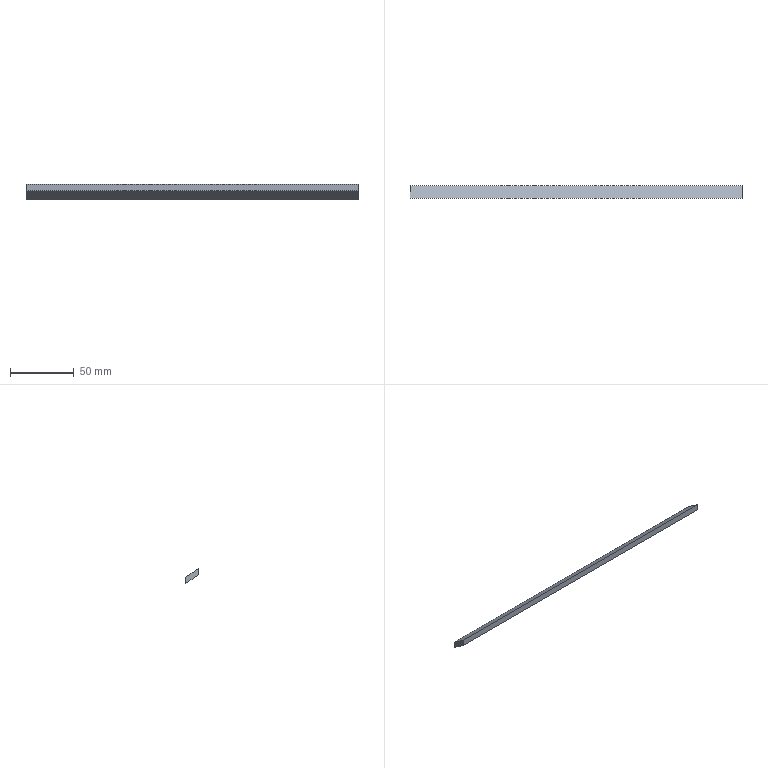Part | STEP file | 06-30 Up-down dovetail press strip | 1 solid | 6 faces | box 260 x 10 x 12.002 mm | volume 13000 mm3 | plane 6
STEP:
#1=CARTESIAN_POINT('',(0.,0.,0.));
#2=DIRECTION('',(0.,0.,1.));
#3=DIRECTION('',(1.,0.,0.));
#4=AXIS2_PLACEMENT_3D('',#1,#2,#3);
#5=CARTESIAN_POINT('',(260.,0.,-0.000000002));
#6=VERTEX_POINT('',#5);
#7=CARTESIAN_POINT('',(0.,0.,-0.000000001));
#8=VERTEX_POINT('',#7);
#9=CARTESIAN_POINT('',(130.,0.,0.));
#10=DIRECTION('',(-1.,0.,0.));
#11=VECTOR('',#10,1.);
#12=LINE('',#9,#11);
#13=CARTESIAN_POINT('',(0.,0.,0.));
#14=DIRECTION('',(0.,-0.5736,-0.8192));
#15=DIRECTION('',(0.,0.8192,-0.5736));
#16=AXIS2_PLACEMENT_3D('',#13,#14,#15);
#17=PLANE('',#16);
#18=CARTESIAN_POINT('',(0.,130.));
#19=DIRECTION('',(0.,-1.));
#20=VECTOR('',#19,1.);
#21=LINE('',#18,#20);
#22=(GEOMETRIC_REPRESENTATION_CONTEXT(2)PARAMETRIC_REPRESENTATION_CONTEXT()REPRESENTATION_CONTEXT('',''));
#23=DEFINITIONAL_REPRESENTATION('',(#21),#22);
#24=PCURVE('',#17,#23);
#25=CARTESIAN_POINT('',(0.,0.,-5.));
#26=DIRECTION('',(0.,1.,0.));
#27=DIRECTION('',(0.,0.,1.));
#28=AXIS2_PLACEMENT_3D('',#25,#26,#27);
#29=PLANE('',#28);
#30=CARTESIAN_POINT('',(5.,130.));
#31=DIRECTION('',(0.,-1.));
#32=VECTOR('',#31,1.);
#33=LINE('',#30,#32);
#34=(GEOMETRIC_REPRESENTATION_CONTEXT(2)PARAMETRIC_REPRESENTATION_CONTEXT()REPRESENTATION_CONTEXT('',''));
#35=DEFINITIONAL_REPRESENTATION('',(#33),#34);
#36=PCURVE('',#29,#35);
#37=SURFACE_CURVE('',#12,(#24,#36),.PCURVE_S1.);
#38=EDGE_CURVE('',#6,#8,#37,.T.);
#39=ORIENTED_EDGE('',*,*,#38,.F.);
#40=CARTESIAN_POINT('',(260.,10.,-7.002));
#41=VERTEX_POINT('',#40);
#42=CARTESIAN_POINT('',(260.,5.,-3.501));
#43=DIRECTION('',(0.,-0.8192,0.5736));
#44=VECTOR('',#43,1.);
#45=LINE('',#42,#44);
#46=CARTESIAN_POINT('',(6.104,260.));
#47=DIRECTION('',(-1.,0.));
#48=VECTOR('',#47,1.);
#49=LINE('',#46,#48);
#50=(GEOMETRIC_REPRESENTATION_CONTEXT(2)PARAMETRIC_REPRESENTATION_CONTEXT()REPRESENTATION_CONTEXT('',''));
#51=DEFINITIONAL_REPRESENTATION('',(#49),#50);
#52=PCURVE('',#17,#51);
#53=CARTESIAN_POINT('',(260.,0.,0.07201));
#54=DIRECTION('',(1.,0.,0.));
#55=DIRECTION('',(0.,0.,-1.));
#56=AXIS2_PLACEMENT_3D('',#53,#54,#55);
#57=PLANE('',#56);
#58=CARTESIAN_POINT('',(3.573,5.));
#59=DIRECTION('',(-0.5736,-0.8192));
#60=VECTOR('',#59,1.);
#61=LINE('',#58,#60);
#62=(GEOMETRIC_REPRESENTATION_CONTEXT(2)PARAMETRIC_REPRESENTATION_CONTEXT()REPRESENTATION_CONTEXT('',''));
#63=DEFINITIONAL_REPRESENTATION('',(#61),#62);
#64=PCURVE('',#57,#63);
#65=SURFACE_CURVE('',#45,(#52,#64),.PCURVE_S1.);
#66=EDGE_CURVE('',#41,#6,#65,.T.);
#67=ORIENTED_EDGE('',*,*,#66,.F.);
#68=CARTESIAN_POINT('',(0.,10.,-7.002));
#69=VERTEX_POINT('',#68);
#70=CARTESIAN_POINT('',(130.,10.,-7.002));
#71=DIRECTION('',(1.,0.,0.));
#72=VECTOR('',#71,1.);
#73=LINE('',#70,#72);
#74=CARTESIAN_POINT('',(12.208,130.));
#75=DIRECTION('',(0.,1.));
#76=VECTOR('',#75,1.);
#77=LINE('',#74,#76);
#78=(GEOMETRIC_REPRESENTATION_CONTEXT(2)PARAMETRIC_REPRESENTATION_CONTEXT()REPRESENTATION_CONTEXT('',''));
#79=DEFINITIONAL_REPRESENTATION('',(#77),#78);
#80=PCURVE('',#17,#79);
#81=CARTESIAN_POINT('',(0.,10.,-7.002));
#82=DIRECTION('',(0.,-1.,0.));
#83=DIRECTION('',(0.,0.,-1.));
#84=AXIS2_PLACEMENT_3D('',#81,#82,#83);
#85=PLANE('',#84);
#86=CARTESIAN_POINT('',(0.,130.));
#87=DIRECTION('',(0.,1.));
#88=VECTOR('',#87,1.);
#89=LINE('',#86,#88);
#90=(GEOMETRIC_REPRESENTATION_CONTEXT(2)PARAMETRIC_REPRESENTATION_CONTEXT()REPRESENTATION_CONTEXT('',''));
#91=DEFINITIONAL_REPRESENTATION('',(#89),#90);
#92=PCURVE('',#85,#91);
#93=SURFACE_CURVE('',#73,(#80,#92),.PCURVE_S1.);
#94=EDGE_CURVE('',#69,#41,#93,.T.);
#95=ORIENTED_EDGE('',*,*,#94,.F.);
#96=CARTESIAN_POINT('',(0.,5.,-3.501));
#97=DIRECTION('',(0.,0.8192,-0.5736));
#98=VECTOR('',#97,1.);
#99=LINE('',#96,#98);
#100=CARTESIAN_POINT('',(6.104,0.));
#101=DIRECTION('',(1.,0.));
#102=VECTOR('',#101,1.);
#103=LINE('',#100,#102);
#104=(GEOMETRIC_REPRESENTATION_CONTEXT(2)PARAMETRIC_REPRESENTATION_CONTEXT()REPRESENTATION_CONTEXT('',''));
#105=DEFINITIONAL_REPRESENTATION('',(#103),#104);
#106=PCURVE('',#17,#105);
#107=CARTESIAN_POINT('',(0.,0.,0.07201));
#108=DIRECTION('',(1.,0.,0.));
#109=DIRECTION('',(0.,0.,-1.));
#110=AXIS2_PLACEMENT_3D('',#107,#108,#109);
#111=PLANE('',#110);
#112=CARTESIAN_POINT('',(3.573,5.));
#113=DIRECTION('',(0.5736,0.8192));
#114=VECTOR('',#113,1.);
#115=LINE('',#112,#114);
#116=(GEOMETRIC_REPRESENTATION_CONTEXT(2)PARAMETRIC_REPRESENTATION_CONTEXT()REPRESENTATION_CONTEXT('',''));
#117=DEFINITIONAL_REPRESENTATION('',(#115),#116);
#118=PCURVE('',#111,#117);
#119=SURFACE_CURVE('',#99,(#106,#118),.PCURVE_S1.);
#120=EDGE_CURVE('',#8,#69,#119,.T.);
#121=ORIENTED_EDGE('',*,*,#120,.F.);
#122=EDGE_LOOP('',(#39,#67,#95,#121));
#123=FACE_BOUND('',#122,.T.);
#124=ADVANCED_FACE('',(#123),#17,.F.);
#125=CARTESIAN_POINT('',(0.,10.,-12.002));
#126=VERTEX_POINT('',#125);
#127=CARTESIAN_POINT('',(0.,10.,-6.001));
#128=DIRECTION('',(0.,0.,1.));
#129=VECTOR('',#128,1.);
#130=LINE('',#127,#129);
#131=CARTESIAN_POINT('',(6.073,10.));
#132=DIRECTION('',(-1.,0.));
#133=VECTOR('',#132,1.);
#134=LINE('',#131,#133);
#135=(GEOMETRIC_REPRESENTATION_CONTEXT(2)PARAMETRIC_REPRESENTATION_CONTEXT()REPRESENTATION_CONTEXT('',''));
#136=DEFINITIONAL_REPRESENTATION('',(#134),#135);
#137=PCURVE('',#111,#136);
#138=CARTESIAN_POINT('',(-1.001,0.));
#139=DIRECTION('',(-1.,0.));
#140=VECTOR('',#139,1.);
#141=LINE('',#138,#140);
#142=(GEOMETRIC_REPRESENTATION_CONTEXT(2)PARAMETRIC_REPRESENTATION_CONTEXT()REPRESENTATION_CONTEXT('',''));
#143=DEFINITIONAL_REPRESENTATION('',(#141),#142);
#144=PCURVE('',#85,#143);
#145=SURFACE_CURVE('',#130,(#137,#144),.PCURVE_S1.);
#146=EDGE_CURVE('',#126,#69,#145,.T.);
#147=ORIENTED_EDGE('',*,*,#146,.F.);
#148=CARTESIAN_POINT('',(0.,0.,-5.));
#149=VERTEX_POINT('',#148);
#150=CARTESIAN_POINT('',(0.,10.,-12.002));
#151=DIRECTION('',(0.,0.8192,-0.5736));
#152=VECTOR('',#151,1.);
#153=LINE('',#150,#152);
#154=CARTESIAN_POINT('',(12.074,10.));
#155=DIRECTION('',(0.5736,0.8192));
#156=VECTOR('',#155,1.);
#157=LINE('',#154,#156);
#158=(GEOMETRIC_REPRESENTATION_CONTEXT(2)PARAMETRIC_REPRESENTATION_CONTEXT()REPRESENTATION_CONTEXT('',''));
#159=DEFINITIONAL_REPRESENTATION('',(#157),#158);
#160=PCURVE('',#111,#159);
#161=CARTESIAN_POINT('',(0.,10.,-12.002));
#162=DIRECTION('',(0.,0.5736,0.8192));
#163=DIRECTION('',(0.,-0.8192,0.5736));
#164=AXIS2_PLACEMENT_3D('',#161,#162,#163);
#165=PLANE('',#164);
#166=CARTESIAN_POINT('',(0.,0.));
#167=DIRECTION('',(-1.,0.));
#168=VECTOR('',#167,1.);
#169=LINE('',#166,#168);
#170=(GEOMETRIC_REPRESENTATION_CONTEXT(2)PARAMETRIC_REPRESENTATION_CONTEXT()REPRESENTATION_CONTEXT('',''));
#171=DEFINITIONAL_REPRESENTATION('',(#169),#170);
#172=PCURVE('',#165,#171);
#173=SURFACE_CURVE('',#153,(#160,#172),.PCURVE_S1.);
#174=EDGE_CURVE('',#149,#126,#173,.T.);
#175=ORIENTED_EDGE('',*,*,#174,.F.);
#176=CARTESIAN_POINT('',(0.,0.,-6.001));
#177=DIRECTION('',(0.,0.,-1.));
#178=VECTOR('',#177,1.);
#179=LINE('',#176,#178);
#180=CARTESIAN_POINT('',(6.073,0.));
#181=DIRECTION('',(1.,0.));
#182=VECTOR('',#181,1.);
#183=LINE('',#180,#182);
#184=(GEOMETRIC_REPRESENTATION_CONTEXT(2)PARAMETRIC_REPRESENTATION_CONTEXT()REPRESENTATION_CONTEXT('',''));
#185=DEFINITIONAL_REPRESENTATION('',(#183),#184);
#186=PCURVE('',#111,#185);
#187=CARTESIAN_POINT('',(-1.001,0.));
#188=DIRECTION('',(-1.,0.));
#189=VECTOR('',#188,1.);
#190=LINE('',#187,#189);
#191=(GEOMETRIC_REPRESENTATION_CONTEXT(2)PARAMETRIC_REPRESENTATION_CONTEXT()REPRESENTATION_CONTEXT('',''));
#192=DEFINITIONAL_REPRESENTATION('',(#190),#191);
#193=PCURVE('',#29,#192);
#194=SURFACE_CURVE('',#179,(#186,#193),.PCURVE_S1.);
#195=EDGE_CURVE('',#8,#149,#194,.T.);
#196=ORIENTED_EDGE('',*,*,#195,.F.);
#197=ORIENTED_EDGE('',*,*,#120,.T.);
#198=EDGE_LOOP('',(#147,#175,#196,#197));
#199=FACE_BOUND('',#198,.T.);
#200=ADVANCED_FACE('',(#199),#111,.F.);
#201=CARTESIAN_POINT('',(260.,0.,-5.));
#202=VERTEX_POINT('',#201);
#203=CARTESIAN_POINT('',(130.,0.,-5.));
#204=DIRECTION('',(-1.,0.,0.));
#205=VECTOR('',#204,1.);
#206=LINE('',#203,#205);
#207=CARTESIAN_POINT('',(0.,130.));
#208=DIRECTION('',(0.,-1.));
#209=VECTOR('',#208,1.);
#210=LINE('',#207,#209);
#211=(GEOMETRIC_REPRESENTATION_CONTEXT(2)PARAMETRIC_REPRESENTATION_CONTEXT()REPRESENTATION_CONTEXT('',''));
#212=DEFINITIONAL_REPRESENTATION('',(#210),#211);
#213=PCURVE('',#29,#212);
#214=CARTESIAN_POINT('',(12.208,130.));
#215=DIRECTION('',(0.,-1.));
#216=VECTOR('',#215,1.);
#217=LINE('',#214,#216);
#218=(GEOMETRIC_REPRESENTATION_CONTEXT(2)PARAMETRIC_REPRESENTATION_CONTEXT()REPRESENTATION_CONTEXT('',''));
#219=DEFINITIONAL_REPRESENTATION('',(#217),#218);
#220=PCURVE('',#165,#219);
#221=SURFACE_CURVE('',#206,(#213,#220),.PCURVE_S1.);
#222=EDGE_CURVE('',#202,#149,#221,.T.);
#223=ORIENTED_EDGE('',*,*,#222,.F.);
#224=CARTESIAN_POINT('',(260.,0.,-2.5));
#225=DIRECTION('',(0.,0.,-1.));
#226=VECTOR('',#225,1.);
#227=LINE('',#224,#226);
#228=CARTESIAN_POINT('',(2.5,260.));
#229=DIRECTION('',(-1.,0.));
#230=VECTOR('',#229,1.);
#231=LINE('',#228,#230);
#232=(GEOMETRIC_REPRESENTATION_CONTEXT(2)PARAMETRIC_REPRESENTATION_CONTEXT()REPRESENTATION_CONTEXT('',''));
#233=DEFINITIONAL_REPRESENTATION('',(#231),#232);
#234=PCURVE('',#29,#233);
#235=CARTESIAN_POINT('',(2.572,0.));
#236=DIRECTION('',(1.,0.));
#237=VECTOR('',#236,1.);
#238=LINE('',#235,#237);
#239=(GEOMETRIC_REPRESENTATION_CONTEXT(2)PARAMETRIC_REPRESENTATION_CONTEXT()REPRESENTATION_CONTEXT('',''));
#240=DEFINITIONAL_REPRESENTATION('',(#238),#239);
#241=PCURVE('',#57,#240);
#242=SURFACE_CURVE('',#227,(#234,#241),.PCURVE_S1.);
#243=EDGE_CURVE('',#6,#202,#242,.T.);
#244=ORIENTED_EDGE('',*,*,#243,.F.);
#245=ORIENTED_EDGE('',*,*,#38,.T.);
#246=ORIENTED_EDGE('',*,*,#195,.T.);
#247=EDGE_LOOP('',(#223,#244,#245,#246));
#248=FACE_BOUND('',#247,.T.);
#249=ADVANCED_FACE('',(#248),#29,.F.);
#250=CARTESIAN_POINT('',(260.,10.,-12.002));
#251=VERTEX_POINT('',#250);
#252=CARTESIAN_POINT('',(260.,0.,-5.));
#253=DIRECTION('',(0.,0.8192,-0.5736));
#254=VECTOR('',#253,1.);
#255=LINE('',#252,#254);
#256=CARTESIAN_POINT('',(5.072,0.));
#257=DIRECTION('',(0.5736,0.8192));
#258=VECTOR('',#257,1.);
#259=LINE('',#256,#258);
#260=(GEOMETRIC_REPRESENTATION_CONTEXT(2)PARAMETRIC_REPRESENTATION_CONTEXT()REPRESENTATION_CONTEXT('',''));
#261=DEFINITIONAL_REPRESENTATION('',(#259),#260);
#262=PCURVE('',#57,#261);
#263=CARTESIAN_POINT('',(12.208,260.));
#264=DIRECTION('',(-1.,0.));
#265=VECTOR('',#264,1.);
#266=LINE('',#263,#265);
#267=(GEOMETRIC_REPRESENTATION_CONTEXT(2)PARAMETRIC_REPRESENTATION_CONTEXT()REPRESENTATION_CONTEXT('',''));
#268=DEFINITIONAL_REPRESENTATION('',(#266),#267);
#269=PCURVE('',#165,#268);
#270=SURFACE_CURVE('',#255,(#262,#269),.PCURVE_S1.);
#271=EDGE_CURVE('',#202,#251,#270,.T.);
#272=ORIENTED_EDGE('',*,*,#271,.T.);
#273=CARTESIAN_POINT('',(260.,10.,-6.001));
#274=DIRECTION('',(0.,0.,1.));
#275=VECTOR('',#274,1.);
#276=LINE('',#273,#275);
#277=CARTESIAN_POINT('',(6.073,10.));
#278=DIRECTION('',(-1.,0.));
#279=VECTOR('',#278,1.);
#280=LINE('',#277,#279);
#281=(GEOMETRIC_REPRESENTATION_CONTEXT(2)PARAMETRIC_REPRESENTATION_CONTEXT()REPRESENTATION_CONTEXT('',''));
#282=DEFINITIONAL_REPRESENTATION('',(#280),#281);
#283=PCURVE('',#57,#282);
#284=CARTESIAN_POINT('',(-1.001,260.));
#285=DIRECTION('',(-1.,0.));
#286=VECTOR('',#285,1.);
#287=LINE('',#284,#286);
#288=(GEOMETRIC_REPRESENTATION_CONTEXT(2)PARAMETRIC_REPRESENTATION_CONTEXT()REPRESENTATION_CONTEXT('',''));
#289=DEFINITIONAL_REPRESENTATION('',(#287),#288);
#290=PCURVE('',#85,#289);
#291=SURFACE_CURVE('',#276,(#283,#290),.PCURVE_S1.);
#292=EDGE_CURVE('',#251,#41,#291,.T.);
#293=ORIENTED_EDGE('',*,*,#292,.T.);
#294=ORIENTED_EDGE('',*,*,#66,.T.);
#295=ORIENTED_EDGE('',*,*,#243,.T.);
#296=EDGE_LOOP('',(#272,#293,#294,#295));
#297=FACE_BOUND('',#296,.T.);
#298=ADVANCED_FACE('',(#297),#57,.T.);
#299=ORIENTED_EDGE('',*,*,#94,.T.);
#300=ORIENTED_EDGE('',*,*,#292,.F.);
#301=CARTESIAN_POINT('',(130.,10.,-12.002));
#302=DIRECTION('',(1.,0.,0.));
#303=VECTOR('',#302,1.);
#304=LINE('',#301,#303);
#305=CARTESIAN_POINT('',(5.,130.));
#306=DIRECTION('',(0.,1.));
#307=VECTOR('',#306,1.);
#308=LINE('',#305,#307);
#309=(GEOMETRIC_REPRESENTATION_CONTEXT(2)PARAMETRIC_REPRESENTATION_CONTEXT()REPRESENTATION_CONTEXT('',''));
#310=DEFINITIONAL_REPRESENTATION('',(#308),#309);
#311=PCURVE('',#85,#310);
#312=CARTESIAN_POINT('',(0.,130.));
#313=DIRECTION('',(0.,1.));
#314=VECTOR('',#313,1.);
#315=LINE('',#312,#314);
#316=(GEOMETRIC_REPRESENTATION_CONTEXT(2)PARAMETRIC_REPRESENTATION_CONTEXT()REPRESENTATION_CONTEXT('',''));
#317=DEFINITIONAL_REPRESENTATION('',(#315),#316);
#318=PCURVE('',#165,#317);
#319=SURFACE_CURVE('',#304,(#311,#318),.PCURVE_S1.);
#320=EDGE_CURVE('',#126,#251,#319,.T.);
#321=ORIENTED_EDGE('',*,*,#320,.F.);
#322=ORIENTED_EDGE('',*,*,#146,.T.);
#323=EDGE_LOOP('',(#299,#300,#321,#322));
#324=FACE_BOUND('',#323,.T.);
#325=ADVANCED_FACE('',(#324),#85,.F.);
#326=ORIENTED_EDGE('',*,*,#320,.T.);
#327=ORIENTED_EDGE('',*,*,#271,.F.);
#328=ORIENTED_EDGE('',*,*,#222,.T.);
#329=ORIENTED_EDGE('',*,*,#174,.T.);
#330=EDGE_LOOP('',(#326,#327,#328,#329));
#331=FACE_BOUND('',#330,.T.);
#332=ADVANCED_FACE('',(#331),#165,.F.);
#333=CLOSED_SHELL('',(#124,#200,#249,#298,#325,#332));
#334=MANIFOLD_SOLID_BREP('',#333);
#335=(LENGTH_UNIT()NAMED_UNIT(*)SI_UNIT(.MILLI.,.METRE.));
#336=UNCERTAINTY_MEASURE_WITH_UNIT(LENGTH_MEASURE(0.0000001),#335,'','');
#337=(NAMED_UNIT(*)PLANE_ANGLE_UNIT()SI_UNIT($,.RADIAN.));
#338=(NAMED_UNIT(*)SI_UNIT($,.STERADIAN.)SOLID_ANGLE_UNIT());
#339=(GEOMETRIC_REPRESENTATION_CONTEXT(3)GLOBAL_UNCERTAINTY_ASSIGNED_CONTEXT((#336))GLOBAL_UNIT_ASSIGNED_CONTEXT((#335,#337,#338))REPRESENTATION_CONTEXT('',''));
#340=ADVANCED_BREP_SHAPE_REPRESENTATION('',(#4,#334),#339);